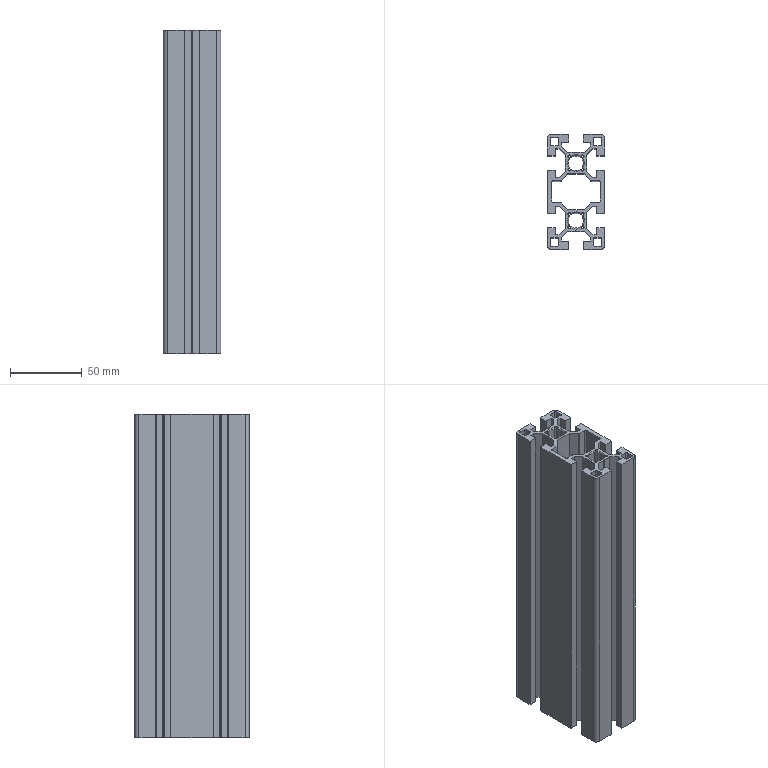Part | STEP file | 0245_015_HFS8-4080-225-LTP | 1 solid | 204 faces | box 40 x 80 x 225 mm | volume 250637 mm3 | plane 112 | cylinder 82 | cone 10 | commonest cylinder face diameters 2 x36 0.762 x20 0.6 x12 10.5 x10 6 x4